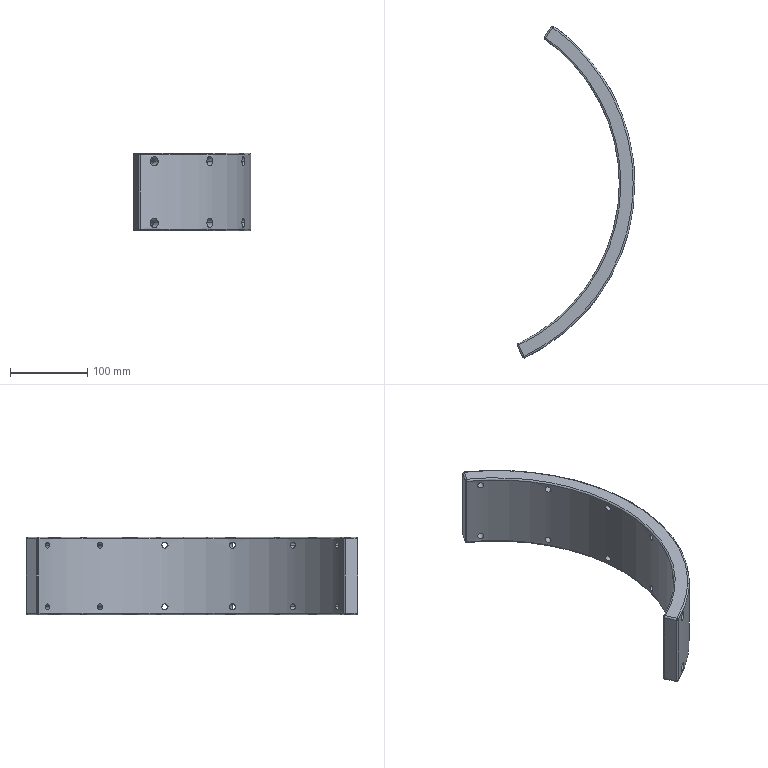Part | SolidWorks | features CirPattern 1, Cut 1, Extrusion 1, Fillet 1, MirrorPattern 1, RefAxis 1, RevCut 1 | 1 solid | 80 faces | box 152.144 x 429.908 x 100 mm | volume 988120 mm3 | cylinder 36 | cone 24 | torus 8 | sphere 8 | plane 4 | commonest cylinder face diameters 8 x24 4 x10 460 x1 500 x1